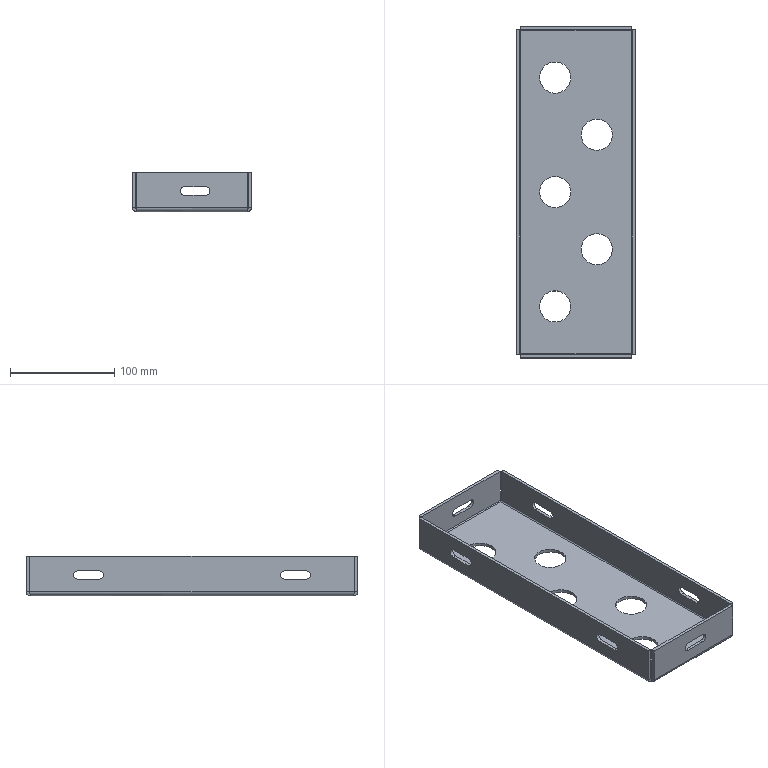Part | NX | features BREP 1 | 1 solid | 72 faces | box 114.1 x 319 x 38 mm | volume 179476 mm3 | plane 34 | cylinder 30 | spline 8 | commonest cylinder face diameters 8.5 x12 30 x10 2 x4 8 x4